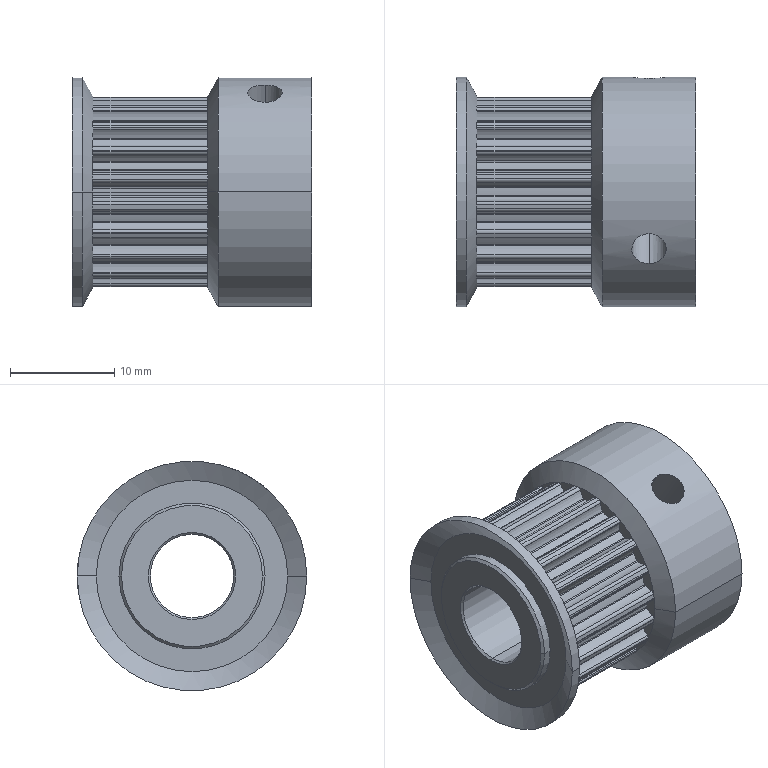Part | SolidWorks | features BaseBody 1 | 1 solid | 248 faces | box 23 x 22 x 22 mm | volume 5516 mm3 | cylinder 193 | plane 43 | cone 12 | commonest cylinder face diameters 0.56 x54 0.3 x44 3.95 x42 16.12 x21 18.34 x20 3.3 x4